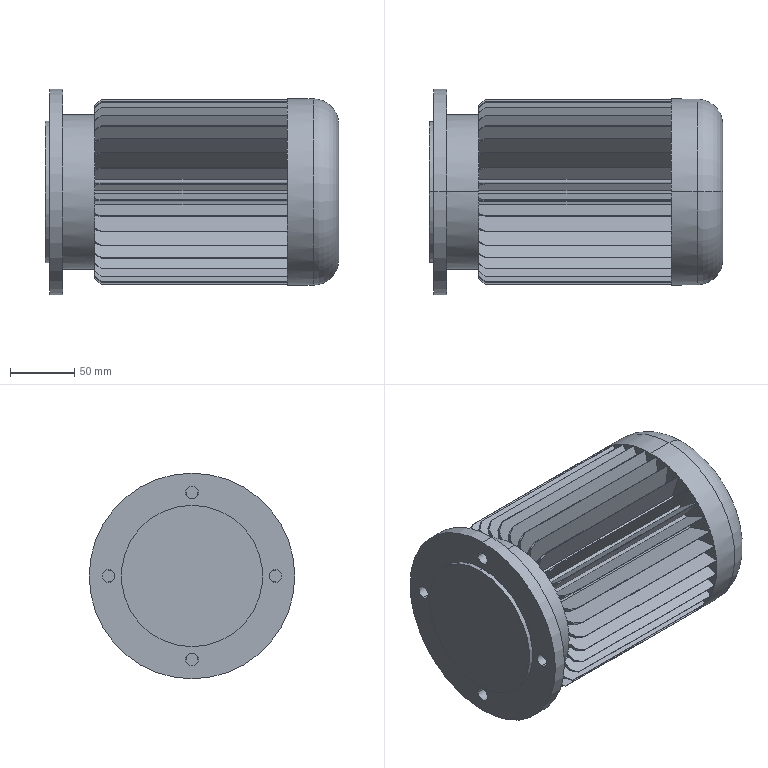Part | SolidWorks | features CirPattern 2, ICE 2, Chamfer 1, Fillet 1, Revolution 1 | 1 solid | 274 faces | box 228.5 x 160 x 160 mm | volume 2710519 mm3 | plane 220 | cone 36 | cylinder 16 | torus 2 | commonest cylinder face diameters 10 x8 110 x2 120 x2 145 x2 160 x2